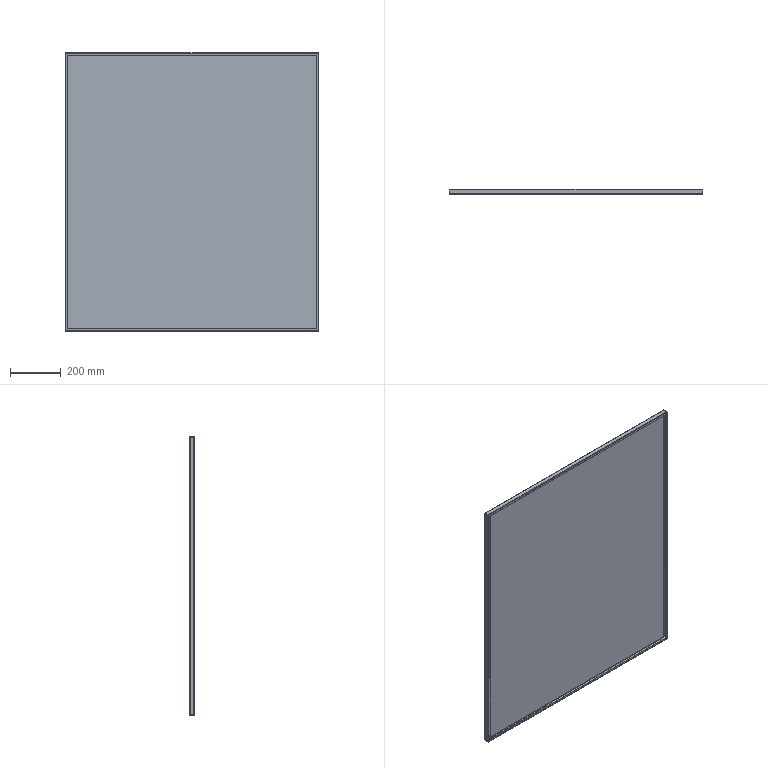Part | SolidWorks | features EdgeFlange 2, FlatPattern 1, SMBaseFlange 1, SheetMetal 1 | 1 solid | 70 faces | box 997 x 20 x 1097 mm | volume 1801010 mm3 | plane 38 | spline 16 | cylinder 16 | commonest cylinder face diameters 1.473 x8 4.473 x8